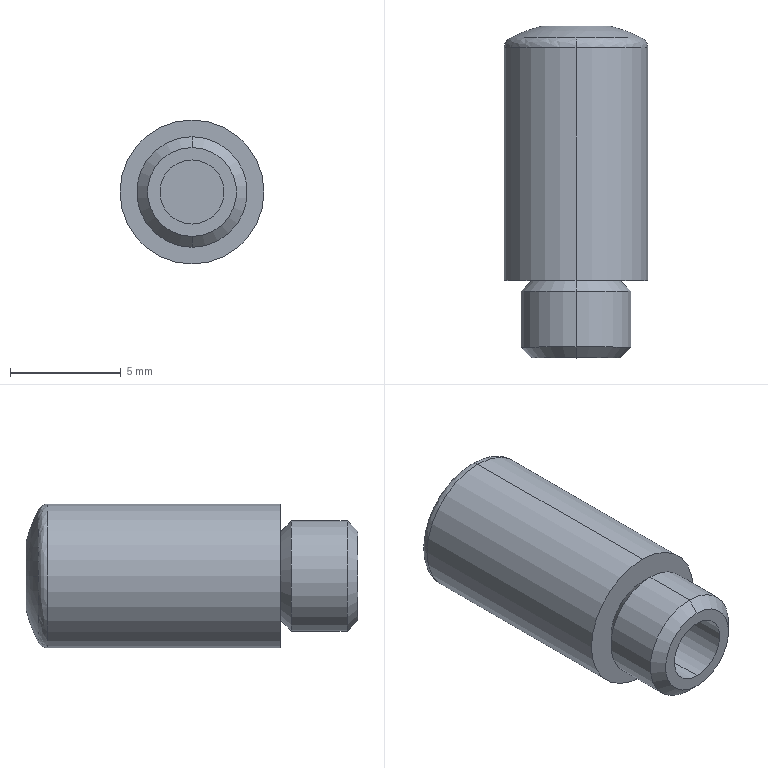Part | SolidWorks | features BaseBody 1 | 1 solid | 18 faces | box 6.5 x 15 x 6.5 mm | volume 404.686 mm3 | cylinder 6 | spline 4 | cone 4 | plane 4 | commonest cylinder face diameters 2.9 x2 5 x2 6.5 x2
STEP:
#1=CARTESIAN_POINT('',(-2.979,10.957,0.));
#2=VERTEX_POINT('',#1);
#3=CARTESIAN_POINT('',(0.,10.957,-2.979));
#4=VERTEX_POINT('',#3);
#5=CARTESIAN_POINT('',(0.,10.957,0.));
#6=DIRECTION('',(0.,-1.,0.));
#7=DIRECTION('',(0.,0.,1.));
#8=AXIS2_PLACEMENT_3D('',#5,#6,#7);
#9=CIRCLE('',#8,2.979);
#10=EDGE_CURVE('',#2,#4,#9,.T.);
#11=ORIENTED_EDGE('',*,*,#10,.T.);
#12=CARTESIAN_POINT('',(0.,10.513,-3.25));
#13=VERTEX_POINT('',#12);
#14=CARTESIAN_POINT('',(0.,10.513,-2.75));
#15=DIRECTION('',(-1.,0.,0.));
#16=DIRECTION('',(0.,0.,-1.));
#17=AXIS2_PLACEMENT_3D('',#14,#15,#16);
#18=CIRCLE('',#17,0.5);
#19=EDGE_CURVE('',#4,#13,#18,.T.);
#20=ORIENTED_EDGE('',*,*,#19,.T.);
#21=CARTESIAN_POINT('',(0.,10.513,3.25));
#22=VERTEX_POINT('',#21);
#23=CARTESIAN_POINT('',(0.,10.513,0.));
#24=DIRECTION('',(0.,-1.,0.));
#25=DIRECTION('',(0.,0.,-1.));
#26=AXIS2_PLACEMENT_3D('',#23,#24,#25);
#27=CIRCLE('',#26,3.25);
#28=EDGE_CURVE('',#22,#13,#27,.T.);
#29=ORIENTED_EDGE('',*,*,#28,.F.);
#30=CARTESIAN_POINT('',(0.,10.957,2.979));
#31=VERTEX_POINT('',#30);
#32=CARTESIAN_POINT('',(0.,10.513,2.75));
#33=DIRECTION('',(1.,0.,0.));
#34=DIRECTION('',(0.,0.,1.));
#35=AXIS2_PLACEMENT_3D('',#32,#33,#34);
#36=CIRCLE('',#35,0.5);
#37=EDGE_CURVE('',#31,#22,#36,.T.);
#38=ORIENTED_EDGE('',*,*,#37,.F.);
#39=CARTESIAN_POINT('',(0.,10.957,0.));
#40=DIRECTION('',(0.,-1.,0.));
#41=DIRECTION('',(0.,0.,1.));
#42=AXIS2_PLACEMENT_3D('',#39,#40,#41);
#43=CIRCLE('',#42,2.979);
#44=EDGE_CURVE('',#31,#2,#43,.T.);
#45=ORIENTED_EDGE('',*,*,#44,.T.);
#46=EDGE_LOOP('',(#11,#20,#29,#38,#45));
#47=FACE_OUTER_BOUND('',#46,.T.);
#48=CARTESIAN_POINT('',(0.,10.957,-2.979));
#49=CARTESIAN_POINT('',(-5.958,10.957,-2.979));
#50=CARTESIAN_POINT('',(-5.958,10.957,2.979));
#51=CARTESIAN_POINT('',(0.,10.957,2.979));
#52=CARTESIAN_POINT('',(0.,10.869,-3.15));
#53=CARTESIAN_POINT('',(-6.3,10.869,-3.15));
#54=CARTESIAN_POINT('',(-6.3,10.869,3.15));
#55=CARTESIAN_POINT('',(0.,10.869,3.15));
#56=CARTESIAN_POINT('',(0.,10.705,-3.25));
#57=CARTESIAN_POINT('',(-6.5,10.705,-3.25));
#58=CARTESIAN_POINT('',(-6.5,10.705,3.25));
#59=CARTESIAN_POINT('',(0.,10.705,3.25));
#60=CARTESIAN_POINT('',(0.,10.513,-3.25));
#61=CARTESIAN_POINT('',(-6.5,10.513,-3.25));
#62=CARTESIAN_POINT('',(-6.5,10.513,3.25));
#63=CARTESIAN_POINT('',(0.,10.513,3.25));
#64=(BOUNDED_SURFACE()B_SPLINE_SURFACE(3,3,((#48,#49,#50,#51),(#52,#53,#54,#55),(#56,#57,#58,#59),(#60,#61,#62,#63)),.UNSPECIFIED.,.F.,.F.,.F.)B_SPLINE_SURFACE_WITH_KNOTS((4,4),(4,4),(0.,1.),(0.,1.),.UNSPECIFIED.)GEOMETRIC_REPRESENTATION_ITEM()RATIONAL_B_SPLINE_SURFACE(((1.,0.3333,0.3333,1.),(0.9026,0.3009,0.3009,0.9026),(0.9026,0.3009,0.3009,0.9026),(1.,0.3333,0.3333,1.)))REPRESENTATION_ITEM('')SURFACE());
#65=ADVANCED_FACE('',(#47),#64,.T.);
#66=CARTESIAN_POINT('',(2.979,10.957,0.));
#67=VERTEX_POINT('',#66);
#68=CARTESIAN_POINT('',(0.,10.957,0.));
#69=DIRECTION('',(0.,-1.,0.));
#70=DIRECTION('',(0.,0.,1.));
#71=AXIS2_PLACEMENT_3D('',#68,#69,#70);
#72=CIRCLE('',#71,2.979);
#73=EDGE_CURVE('',#67,#31,#72,.T.);
#74=ORIENTED_EDGE('',*,*,#73,.F.);
#75=CARTESIAN_POINT('',(1.519,11.5,0.));
#76=VERTEX_POINT('',#75);
#77=CARTESIAN_POINT('',(0.,5.18,0.));
#78=DIRECTION('',(0.,0.,1.));
#79=DIRECTION('',(1.,0.,0.));
#80=AXIS2_PLACEMENT_3D('',#77,#78,#79);
#81=CIRCLE('',#80,6.5);
#82=EDGE_CURVE('',#67,#76,#81,.T.);
#83=ORIENTED_EDGE('',*,*,#82,.T.);
#84=CARTESIAN_POINT('',(-1.519,11.5,0.));
#85=VERTEX_POINT('',#84);
#86=CARTESIAN_POINT('',(1.519,11.5,0.));
#87=CARTESIAN_POINT('',(1.519,11.5,0.1003));
#88=CARTESIAN_POINT('',(1.509,11.5,0.199));
#89=CARTESIAN_POINT('',(1.471,11.5,0.3931));
#90=CARTESIAN_POINT('',(1.441,11.5,0.4896));
#91=CARTESIAN_POINT('',(1.365,11.5,0.6736));
#92=CARTESIAN_POINT('',(1.319,11.5,0.7608));
#93=CARTESIAN_POINT('',(1.208,11.5,0.9259));
#94=CARTESIAN_POINT('',(1.144,11.5,1.004));
#95=CARTESIAN_POINT('',(0.934,11.5,1.214));
#96=CARTESIAN_POINT('',(0.7645,11.5,1.327));
#97=CARTESIAN_POINT('',(0.399,11.5,1.479));
#98=CARTESIAN_POINT('',(0.1991,11.5,1.519));
#99=CARTESIAN_POINT('',(-0.09803,11.5,1.519));
#100=CARTESIAN_POINT('',(-0.1986,11.5,1.509));
#101=CARTESIAN_POINT('',(-0.3935,11.5,1.471));
#102=CARTESIAN_POINT('',(-0.4882,11.5,1.442));
#103=CARTESIAN_POINT('',(-0.6721,11.5,1.366));
#104=CARTESIAN_POINT('',(-0.761,11.5,1.318));
#105=CARTESIAN_POINT('',(-0.9257,11.5,1.209));
#106=CARTESIAN_POINT('',(-1.002,11.5,1.146));
#107=CARTESIAN_POINT('',(-1.215,11.5,0.9333));
#108=CARTESIAN_POINT('',(-1.327,11.5,0.7661));
#109=CARTESIAN_POINT('',(-1.479,11.5,0.398));
#110=CARTESIAN_POINT('',(-1.519,11.5,0.2007));
#111=CARTESIAN_POINT('',(-1.519,11.5,0.));
#112=B_SPLINE_CURVE_WITH_KNOTS('',3,(#86,#87,#88,#89,#90,#91,#92,#93,#94,#95,#96,#97,#98,#99,#100,#101,#102,#103,#104,#105,#106,#107,#108,#109,#110,#111),.UNSPECIFIED.,.F.,.F.,(4,2,2,2,2,2,2,2,2,2,2,2,4),(0.,0.0002968,0.0005935,0.0008903,0.001187,0.001781,0.002374,0.002671,0.002968,0.003264,0.003561,0.004155,0.004748),.UNSPECIFIED.);
#113=EDGE_CURVE('',#76,#85,#112,.T.);
#114=ORIENTED_EDGE('',*,*,#113,.T.);
#115=CARTESIAN_POINT('',(0.,5.18,0.));
#116=DIRECTION('',(0.,0.,1.));
#117=DIRECTION('',(1.,0.,0.));
#118=AXIS2_PLACEMENT_3D('',#115,#116,#117);
#119=CIRCLE('',#118,6.5);
#120=EDGE_CURVE('',#85,#2,#119,.T.);
#121=ORIENTED_EDGE('',*,*,#120,.T.);
#122=ORIENTED_EDGE('',*,*,#44,.F.);
#123=EDGE_LOOP('',(#74,#83,#114,#121,#122));
#124=FACE_OUTER_BOUND('',#123,.T.);
#125=CARTESIAN_POINT('',(3.012,10.94,0.));
#126=CARTESIAN_POINT('',(3.012,10.94,0.9285));
#127=CARTESIAN_POINT('',(3.012,10.72,1.831));
#128=CARTESIAN_POINT('',(3.012,10.292,2.655));
#129=CARTESIAN_POINT('',(1.087,11.947,0.));
#130=CARTESIAN_POINT('',(1.087,11.947,1.091));
#131=CARTESIAN_POINT('',(1.087,11.688,2.151));
#132=CARTESIAN_POINT('',(1.087,11.185,3.119));
#133=CARTESIAN_POINT('',(-1.087,11.947,0.));
#134=CARTESIAN_POINT('',(-1.087,11.947,1.091));
#135=CARTESIAN_POINT('',(-1.087,11.688,2.151));
#136=CARTESIAN_POINT('',(-1.087,11.185,3.119));
#137=CARTESIAN_POINT('',(-3.012,10.94,0.));
#138=CARTESIAN_POINT('',(-3.012,10.94,0.9285));
#139=CARTESIAN_POINT('',(-3.012,10.72,1.831));
#140=CARTESIAN_POINT('',(-3.012,10.292,2.655));
#141=(BOUNDED_SURFACE()B_SPLINE_SURFACE(3,3,((#125,#126,#127,#128),(#129,#130,#131,#132),(#133,#134,#135,#136),(#137,#138,#139,#140)),.UNSPECIFIED.,.F.,.F.,.F.)B_SPLINE_SURFACE_WITH_KNOTS((4,4),(4,4),(0.,1.),(0.,1.),.UNSPECIFIED.)GEOMETRIC_REPRESENTATION_ITEM()RATIONAL_B_SPLINE_SURFACE(((1.,0.981,0.981,1.),(0.9241,0.9065,0.9065,0.9241),(0.9241,0.9065,0.9065,0.9241),(1.,0.981,0.981,1.)))REPRESENTATION_ITEM('')SURFACE());
#142=ADVANCED_FACE('',(#124),#141,.T.);
#143=CARTESIAN_POINT('',(0.,10.513,0.));
#144=DIRECTION('',(0.,-1.,0.));
#145=DIRECTION('',(0.,0.,-1.));
#146=AXIS2_PLACEMENT_3D('',#143,#144,#145);
#147=CIRCLE('',#146,3.25);
#148=EDGE_CURVE('',#13,#22,#147,.T.);
#149=ORIENTED_EDGE('',*,*,#148,.T.);
#150=CARTESIAN_POINT('',(0.,0.,3.25));
#151=VERTEX_POINT('',#150);
#152=CARTESIAN_POINT('',(0.,5.256,3.25));
#153=DIRECTION('',(0.,-1.,0.));
#154=VECTOR('',#153,1000.);
#155=LINE('',#152,#154);
#156=EDGE_CURVE('',#22,#151,#155,.T.);
#157=ORIENTED_EDGE('',*,*,#156,.T.);
#158=CARTESIAN_POINT('',(0.,0.,-3.25));
#159=VERTEX_POINT('',#158);
#160=CARTESIAN_POINT('',(0.,0.,0.));
#161=DIRECTION('',(0.,1.,0.));
#162=DIRECTION('',(0.,0.,-1.));
#163=AXIS2_PLACEMENT_3D('',#160,#161,#162);
#164=CIRCLE('',#163,3.25);
#165=EDGE_CURVE('',#151,#159,#164,.T.);
#166=ORIENTED_EDGE('',*,*,#165,.T.);
#167=CARTESIAN_POINT('',(0.,5.256,-3.25));
#168=DIRECTION('',(0.,-1.,0.));
#169=VECTOR('',#168,1000.);
#170=LINE('',#167,#169);
#171=EDGE_CURVE('',#13,#159,#170,.T.);
#172=ORIENTED_EDGE('',*,*,#171,.F.);
#173=EDGE_LOOP('',(#149,#157,#166,#172));
#174=FACE_OUTER_BOUND('',#173,.T.);
#175=CARTESIAN_POINT('',(0.,5.256,0.));
#176=DIRECTION('',(0.,-1.,0.));
#177=DIRECTION('',(0.,0.,-1.));
#178=AXIS2_PLACEMENT_3D('',#175,#176,#177);
#179=CYLINDRICAL_SURFACE('',#178,3.25);
#180=ADVANCED_FACE('',(#174),#179,.T.);
#181=CARTESIAN_POINT('',(0.,0.,2.009));
#182=VERTEX_POINT('',#181);
#183=CARTESIAN_POINT('',(0.,0.,-2.009));
#184=VERTEX_POINT('',#183);
#185=CARTESIAN_POINT('',(0.,0.,0.));
#186=DIRECTION('',(0.,1.,0.));
#187=DIRECTION('',(0.,0.,-1.));
#188=AXIS2_PLACEMENT_3D('',#185,#186,#187);
#189=CIRCLE('',#188,2.009);
#190=EDGE_CURVE('',#182,#184,#189,.T.);
#191=ORIENTED_EDGE('',*,*,#190,.F.);
#192=CARTESIAN_POINT('',(0.,-0.4905,2.5));
#193=VERTEX_POINT('',#192);
#194=CARTESIAN_POINT('',(0.,-0.4905,2.5));
#195=DIRECTION('',(0.,-0.7071,0.7071));
#196=VECTOR('',#195,1000.);
#197=LINE('',#194,#196);
#198=EDGE_CURVE('',#182,#193,#197,.T.);
#199=ORIENTED_EDGE('',*,*,#198,.T.);
#200=CARTESIAN_POINT('',(0.,-0.4905,-2.5));
#201=VERTEX_POINT('',#200);
#202=CARTESIAN_POINT('',(0.,-0.4905,0.));
#203=DIRECTION('',(0.,1.,0.));
#204=DIRECTION('',(1.,0.,0.));
#205=AXIS2_PLACEMENT_3D('',#202,#203,#204);
#206=CIRCLE('',#205,2.5);
#207=EDGE_CURVE('',#193,#201,#206,.T.);
#208=ORIENTED_EDGE('',*,*,#207,.T.);
#209=CARTESIAN_POINT('',(0.,-0.4905,-2.5));
#210=DIRECTION('',(0.,-0.7071,-0.7071));
#211=VECTOR('',#210,1000.);
#212=LINE('',#209,#211);
#213=EDGE_CURVE('',#184,#201,#212,.T.);
#214=ORIENTED_EDGE('',*,*,#213,.F.);
#215=EDGE_LOOP('',(#191,#199,#208,#214));
#216=FACE_OUTER_BOUND('',#215,.T.);
#217=CARTESIAN_POINT('',(0.,-0.4905,0.));
#218=DIRECTION('',(0.,-1.,0.));
#219=DIRECTION('',(0.,0.,-1.));
#220=AXIS2_PLACEMENT_3D('',#217,#218,#219);
#221=CONICAL_SURFACE('',#220,2.5,0.7854);
#222=ADVANCED_FACE('',(#216),#221,.T.);
#223=ORIENTED_EDGE('',*,*,#207,.F.);
#224=CARTESIAN_POINT('',(0.,-3.01,2.5));
#225=VERTEX_POINT('',#224);
#226=CARTESIAN_POINT('',(0.,-1.75,2.5));
#227=DIRECTION('',(0.,-1.,0.));
#228=VECTOR('',#227,1000.);
#229=LINE('',#226,#228);
#230=EDGE_CURVE('',#193,#225,#229,.T.);
#231=ORIENTED_EDGE('',*,*,#230,.T.);
#232=CARTESIAN_POINT('',(0.,-3.01,-2.5));
#233=VERTEX_POINT('',#232);
#234=CARTESIAN_POINT('',(0.,-3.01,0.));
#235=DIRECTION('',(0.,1.,0.));
#236=DIRECTION('',(0.,0.,-1.));
#237=AXIS2_PLACEMENT_3D('',#234,#235,#236);
#238=CIRCLE('',#237,2.5);
#239=EDGE_CURVE('',#225,#233,#238,.T.);
#240=ORIENTED_EDGE('',*,*,#239,.T.);
#241=CARTESIAN_POINT('',(0.,-1.75,-2.5));
#242=DIRECTION('',(0.,-1.,0.));
#243=VECTOR('',#242,1000.);
#244=LINE('',#241,#243);
#245=EDGE_CURVE('',#201,#233,#244,.T.);
#246=ORIENTED_EDGE('',*,*,#245,.F.);
#247=EDGE_LOOP('',(#223,#231,#240,#246));
#248=FACE_OUTER_BOUND('',#247,.T.);
#249=CARTESIAN_POINT('',(0.,-1.75,0.));
#250=DIRECTION('',(0.,-1.,0.));
#251=DIRECTION('',(0.,0.,-1.));
#252=AXIS2_PLACEMENT_3D('',#249,#250,#251);
#253=CYLINDRICAL_SURFACE('',#252,2.5);
#254=ADVANCED_FACE('',(#248),#253,.T.);
#255=CARTESIAN_POINT('',(0.,-3.5,2.01));
#256=VERTEX_POINT('',#255);
#257=CARTESIAN_POINT('',(0.,-3.5,-2.01));
#258=VERTEX_POINT('',#257);
#259=CARTESIAN_POINT('',(0.,-3.5,0.));
#260=DIRECTION('',(0.,1.,0.));
#261=DIRECTION('',(0.,0.,1.));
#262=AXIS2_PLACEMENT_3D('',#259,#260,#261);
#263=CIRCLE('',#262,2.01);
#264=EDGE_CURVE('',#256,#258,#263,.T.);
#265=ORIENTED_EDGE('',*,*,#264,.T.);
#266=CARTESIAN_POINT('',(0.,-3.009,-2.5));
#267=DIRECTION('',(0.,0.7071,-0.7071));
#268=VECTOR('',#267,1000.);
#269=LINE('',#266,#268);
#270=EDGE_CURVE('',#258,#233,#269,.T.);
#271=ORIENTED_EDGE('',*,*,#270,.T.);
#272=ORIENTED_EDGE('',*,*,#239,.F.);
#273=CARTESIAN_POINT('',(0.,-3.009,2.5));
#274=DIRECTION('',(0.,0.7071,0.7071));
#275=VECTOR('',#274,1000.);
#276=LINE('',#273,#275);
#277=EDGE_CURVE('',#256,#225,#276,.T.);
#278=ORIENTED_EDGE('',*,*,#277,.F.);
#279=EDGE_LOOP('',(#265,#271,#272,#278));
#280=FACE_OUTER_BOUND('',#279,.T.);
#281=CARTESIAN_POINT('',(0.,-3.009,0.));
#282=DIRECTION('',(0.,1.,0.));
#283=DIRECTION('',(0.,0.,1.));
#284=AXIS2_PLACEMENT_3D('',#281,#282,#283);
#285=CONICAL_SURFACE('',#284,2.5,0.7854);
#286=ADVANCED_FACE('',(#280),#285,.T.);
#287=CARTESIAN_POINT('',(0.,1.5,1.45));
#288=VERTEX_POINT('',#287);
#289=CARTESIAN_POINT('',(0.,1.5,-1.45));
#290=VERTEX_POINT('',#289);
#291=CARTESIAN_POINT('',(0.,1.5,0.));
#292=DIRECTION('',(0.,-1.,0.));
#293=DIRECTION('',(0.,0.,-1.));
#294=AXIS2_PLACEMENT_3D('',#291,#292,#293);
#295=CIRCLE('',#294,1.45);
#296=EDGE_CURVE('',#288,#290,#295,.T.);
#297=ORIENTED_EDGE('',*,*,#296,.F.);
#298=CARTESIAN_POINT('',(0.,-3.5,1.45));
#299=VERTEX_POINT('',#298);
#300=CARTESIAN_POINT('',(0.,-1.,1.45));
#301=DIRECTION('',(0.,-1.,0.));
#302=VECTOR('',#301,1000.);
#303=LINE('',#300,#302);
#304=EDGE_CURVE('',#288,#299,#303,.T.);
#305=ORIENTED_EDGE('',*,*,#304,.T.);
#306=CARTESIAN_POINT('',(0.,-3.5,-1.45));
#307=VERTEX_POINT('',#306);
#308=CARTESIAN_POINT('',(0.,-3.5,0.));
#309=DIRECTION('',(0.,1.,0.));
#310=DIRECTION('',(0.,0.,-1.));
#311=AXIS2_PLACEMENT_3D('',#308,#309,#310);
#312=CIRCLE('',#311,1.45);
#313=EDGE_CURVE('',#307,#299,#312,.T.);
#314=ORIENTED_EDGE('',*,*,#313,.F.);
#315=CARTESIAN_POINT('',(0.,-1.,-1.45));
#316=DIRECTION('',(0.,-1.,0.));
#317=VECTOR('',#316,1000.);
#318=LINE('',#315,#317);
#319=EDGE_CURVE('',#290,#307,#318,.T.);
#320=ORIENTED_EDGE('',*,*,#319,.F.);
#321=EDGE_LOOP('',(#297,#305,#314,#320));
#322=FACE_OUTER_BOUND('',#321,.T.);
#323=CARTESIAN_POINT('',(0.,-1.,0.));
#324=DIRECTION('',(0.,-1.,0.));
#325=DIRECTION('',(0.,0.,-1.));
#326=AXIS2_PLACEMENT_3D('',#323,#324,#325);
#327=CYLINDRICAL_SURFACE('',#326,1.45);
#328=ADVANCED_FACE('',(#322),#327,.F.);
#329=ORIENTED_EDGE('',*,*,#156,.F.);
#330=ORIENTED_EDGE('',*,*,#28,.T.);
#331=ORIENTED_EDGE('',*,*,#171,.T.);
#332=CARTESIAN_POINT('',(0.,0.,0.));
#333=DIRECTION('',(0.,1.,0.));
#334=DIRECTION('',(0.,0.,-1.));
#335=AXIS2_PLACEMENT_3D('',#332,#333,#334);
#336=CIRCLE('',#335,3.25);
#337=EDGE_CURVE('',#159,#151,#336,.T.);
#338=ORIENTED_EDGE('',*,*,#337,.T.);
#339=EDGE_LOOP('',(#329,#330,#331,#338));
#340=FACE_OUTER_BOUND('',#339,.T.);
#341=CARTESIAN_POINT('',(0.,5.256,0.));
#342=DIRECTION('',(0.,-1.,0.));
#343=DIRECTION('',(0.,0.,-1.));
#344=AXIS2_PLACEMENT_3D('',#341,#342,#343);
#345=CYLINDRICAL_SURFACE('',#344,3.25);
#346=ADVANCED_FACE('',(#340),#345,.T.);
#347=ORIENTED_EDGE('',*,*,#19,.F.);
#348=CARTESIAN_POINT('',(0.,10.957,0.));
#349=DIRECTION('',(0.,-1.,0.));
#350=DIRECTION('',(0.,0.,1.));
#351=AXIS2_PLACEMENT_3D('',#348,#349,#350);
#352=CIRCLE('',#351,2.979);
#353=EDGE_CURVE('',#4,#67,#352,.T.);
#354=ORIENTED_EDGE('',*,*,#353,.T.);
#355=ORIENTED_EDGE('',*,*,#73,.T.);
#356=ORIENTED_EDGE('',*,*,#37,.T.);
#357=ORIENTED_EDGE('',*,*,#148,.F.);
#358=EDGE_LOOP('',(#347,#354,#355,#356,#357));
#359=FACE_OUTER_BOUND('',#358,.T.);
#360=CARTESIAN_POINT('',(0.,10.957,2.979));
#361=CARTESIAN_POINT('',(5.958,10.957,2.979));
#362=CARTESIAN_POINT('',(5.958,10.957,-2.979));
#363=CARTESIAN_POINT('',(0.,10.957,-2.979));
#364=CARTESIAN_POINT('',(0.,10.869,3.15));
#365=CARTESIAN_POINT('',(6.3,10.869,3.15));
#366=CARTESIAN_POINT('',(6.3,10.869,-3.15));
#367=CARTESIAN_POINT('',(0.,10.869,-3.15));
#368=CARTESIAN_POINT('',(0.,10.705,3.25));
#369=CARTESIAN_POINT('',(6.5,10.705,3.25));
#370=CARTESIAN_POINT('',(6.5,10.705,-3.25));
#371=CARTESIAN_POINT('',(0.,10.705,-3.25));
#372=CARTESIAN_POINT('',(0.,10.513,3.25));
#373=CARTESIAN_POINT('',(6.5,10.513,3.25));
#374=CARTESIAN_POINT('',(6.5,10.513,-3.25));
#375=CARTESIAN_POINT('',(0.,10.513,-3.25));
#376=(BOUNDED_SURFACE()B_SPLINE_SURFACE(3,3,((#360,#361,#362,#363),(#364,#365,#366,#367),(#368,#369,#370,#371),(#372,#373,#374,#375)),.UNSPECIFIED.,.F.,.F.,.T.)B_SPLINE_SURFACE_WITH_KNOTS((4,4),(4,4),(0.,1.),(0.,1.),.UNSPECIFIED.)GEOMETRIC_REPRESENTATION_ITEM()RATIONAL_B_SPLINE_SURFACE(((1.,0.3333,0.3333,1.),(0.9026,0.3009,0.3009,0.9026),(0.9026,0.3009,0.3009,0.9026),(1.,0.3333,0.3333,1.)))REPRESENTATION_ITEM('')SURFACE());
#377=ADVANCED_FACE('',(#359),#376,.T.);
#378=CARTESIAN_POINT('',(0.,0.,0.));
#379=DIRECTION('',(0.,1.,0.));
#380=DIRECTION('',(0.,0.,-1.));
#381=AXIS2_PLACEMENT_3D('',#378,#379,#380);
#382=CIRCLE('',#381,2.009);
#383=EDGE_CURVE('',#184,#182,#382,.T.);
#384=ORIENTED_EDGE('',*,*,#383,.T.);
#385=ORIENTED_EDGE('',*,*,#190,.T.);
#386=EDGE_LOOP('',(#384,#385));
#387=FACE_BOUND('',#386,.T.);
#388=ORIENTED_EDGE('',*,*,#337,.F.);
#389=ORIENTED_EDGE('',*,*,#165,.F.);
#390=EDGE_LOOP('',(#388,#389));
#391=FACE_OUTER_BOUND('',#390,.T.);
#392=CARTESIAN_POINT('',(2.63,0.,0.));
#393=DIRECTION('',(0.,-1.,0.));
#394=DIRECTION('',(0.,0.,-1.));
#395=AXIS2_PLACEMENT_3D('',#392,#393,#394);
#396=PLANE('',#395);
#397=ADVANCED_FACE('',(#387,#391),#396,.T.);
#398=ORIENTED_EDGE('',*,*,#82,.F.);
#399=ORIENTED_EDGE('',*,*,#353,.F.);
#400=ORIENTED_EDGE('',*,*,#10,.F.);
#401=ORIENTED_EDGE('',*,*,#120,.F.);
#402=CARTESIAN_POINT('',(-1.519,11.5,0.));
#403=CARTESIAN_POINT('',(-1.519,11.5,-0.1003));
#404=CARTESIAN_POINT('',(-1.509,11.5,-0.199));
#405=CARTESIAN_POINT('',(-1.471,11.5,-0.3931));
#406=CARTESIAN_POINT('',(-1.441,11.5,-0.4896));
#407=CARTESIAN_POINT('',(-1.365,11.5,-0.6736));
#408=CARTESIAN_POINT('',(-1.319,11.5,-0.7608));
#409=CARTESIAN_POINT('',(-1.208,11.5,-0.9259));
#410=CARTESIAN_POINT('',(-1.144,11.5,-1.004));
#411=CARTESIAN_POINT('',(-0.934,11.5,-1.214));
#412=CARTESIAN_POINT('',(-0.7645,11.5,-1.327));
#413=CARTESIAN_POINT('',(-0.399,11.5,-1.479));
#414=CARTESIAN_POINT('',(-0.1991,11.5,-1.519));
#415=CARTESIAN_POINT('',(0.09803,11.5,-1.519));
#416=CARTESIAN_POINT('',(0.1986,11.5,-1.509));
#417=CARTESIAN_POINT('',(0.3935,11.5,-1.471));
#418=CARTESIAN_POINT('',(0.4882,11.5,-1.442));
#419=CARTESIAN_POINT('',(0.6721,11.5,-1.366));
#420=CARTESIAN_POINT('',(0.761,11.5,-1.318));
#421=CARTESIAN_POINT('',(0.9257,11.5,-1.209));
#422=CARTESIAN_POINT('',(1.002,11.5,-1.146));
#423=CARTESIAN_POINT('',(1.215,11.5,-0.9333));
#424=CARTESIAN_POINT('',(1.327,11.5,-0.7661));
#425=CARTESIAN_POINT('',(1.479,11.5,-0.398));
#426=CARTESIAN_POINT('',(1.519,11.5,-0.2007));
#427=CARTESIAN_POINT('',(1.519,11.5,0.));
#428=B_SPLINE_CURVE_WITH_KNOTS('',3,(#402,#403,#404,#405,#406,#407,#408,#409,#410,#411,#412,#413,#414,#415,#416,#417,#418,#419,#420,#421,#422,#423,#424,#425,#426,#427),.UNSPECIFIED.,.F.,.F.,(4,2,2,2,2,2,2,2,2,2,2,2,4),(0.004748,0.005045,0.005342,0.005639,0.005935,0.006529,0.007123,0.007419,0.007716,0.008013,0.00831,0.008903,0.009497),.UNSPECIFIED.);
#429=EDGE_CURVE('',#85,#76,#428,.T.);
#430=ORIENTED_EDGE('',*,*,#429,.T.);
#431=EDGE_LOOP('',(#398,#399,#400,#401,#430));
#432=FACE_OUTER_BOUND('',#431,.T.);
#433=CARTESIAN_POINT('',(3.012,10.292,-2.655));
#434=CARTESIAN_POINT('',(3.012,10.72,-1.831));
#435=CARTESIAN_POINT('',(3.012,10.94,-0.9285));
#436=CARTESIAN_POINT('',(3.012,10.94,0.));
#437=CARTESIAN_POINT('',(1.087,11.185,-3.119));
#438=CARTESIAN_POINT('',(1.087,11.688,-2.151));
#439=CARTESIAN_POINT('',(1.087,11.947,-1.091));
#440=CARTESIAN_POINT('',(1.087,11.947,0.));
#441=CARTESIAN_POINT('',(-1.087,11.185,-3.119));
#442=CARTESIAN_POINT('',(-1.087,11.688,-2.151));
#443=CARTESIAN_POINT('',(-1.087,11.947,-1.091));
#444=CARTESIAN_POINT('',(-1.087,11.947,0.));
#445=CARTESIAN_POINT('',(-3.012,10.292,-2.655));
#446=CARTESIAN_POINT('',(-3.012,10.72,-1.831));
#447=CARTESIAN_POINT('',(-3.012,10.94,-0.9285));
#448=CARTESIAN_POINT('',(-3.012,10.94,0.));
#449=(BOUNDED_SURFACE()B_SPLINE_SURFACE(3,3,((#433,#434,#435,#436),(#437,#438,#439,#440),(#441,#442,#443,#444),(#445,#446,#447,#448)),.UNSPECIFIED.,.F.,.F.,.F.)B_SPLINE_SURFACE_WITH_KNOTS((4,4),(4,4),(0.,1.),(0.,1.),.UNSPECIFIED.)GEOMETRIC_REPRESENTATION_ITEM()RATIONAL_B_SPLINE_SURFACE(((1.,0.981,0.981,1.),(0.9241,0.9065,0.9065,0.9241),(0.9241,0.9065,0.9065,0.9241),(1.,0.981,0.981,1.)))REPRESENTATION_ITEM('')SURFACE());
#450=ADVANCED_FACE('',(#432),#449,.T.);
#451=ORIENTED_EDGE('',*,*,#198,.F.);
#452=ORIENTED_EDGE('',*,*,#383,.F.);
#453=ORIENTED_EDGE('',*,*,#213,.T.);
#454=CARTESIAN_POINT('',(0.,-0.4905,0.));
#455=DIRECTION('',(0.,1.,0.));
#456=DIRECTION('',(1.,0.,0.));
#457=AXIS2_PLACEMENT_3D('',#454,#455,#456);
#458=CIRCLE('',#457,2.5);
#459=EDGE_CURVE('',#201,#193,#458,.T.);
#460=ORIENTED_EDGE('',*,*,#459,.T.);
#461=EDGE_LOOP('',(#451,#452,#453,#460));
#462=FACE_OUTER_BOUND('',#461,.T.);
#463=CARTESIAN_POINT('',(0.,-0.4905,0.));
#464=DIRECTION('',(0.,-1.,0.));
#465=DIRECTION('',(0.,0.,-1.));
#466=AXIS2_PLACEMENT_3D('',#463,#464,#465);
#467=CONICAL_SURFACE('',#466,2.5,0.7854);
#468=ADVANCED_FACE('',(#462),#467,.T.);
#469=ORIENTED_EDGE('',*,*,#113,.F.);
#470=ORIENTED_EDGE('',*,*,#429,.F.);
#471=EDGE_LOOP('',(#469,#470));
#472=FACE_OUTER_BOUND('',#471,.T.);
#473=CARTESIAN_POINT('',(0.7595,11.5,0.));
#474=DIRECTION('',(0.,1.,0.));
#475=DIRECTION('',(0.,0.,1.));
#476=AXIS2_PLACEMENT_3D('',#473,#474,#475);
#477=PLANE('',#476);
#478=ADVANCED_FACE('',(#472),#477,.T.);
#479=ORIENTED_EDGE('',*,*,#230,.F.);
#480=ORIENTED_EDGE('',*,*,#459,.F.);
#481=ORIENTED_EDGE('',*,*,#245,.T.);
#482=CARTESIAN_POINT('',(0.,-3.01,0.));
#483=DIRECTION('',(0.,1.,0.));
#484=DIRECTION('',(0.,0.,-1.));
#485=AXIS2_PLACEMENT_3D('',#482,#483,#484);
#486=CIRCLE('',#485,2.5);
#487=EDGE_CURVE('',#233,#225,#486,.T.);
#488=ORIENTED_EDGE('',*,*,#487,.T.);
#489=EDGE_LOOP('',(#479,#480,#481,#488));
#490=FACE_OUTER_BOUND('',#489,.T.);
#491=CARTESIAN_POINT('',(0.,-1.75,0.));
#492=DIRECTION('',(0.,-1.,0.));
#493=DIRECTION('',(0.,0.,-1.));
#494=AXIS2_PLACEMENT_3D('',#491,#492,#493);
#495=CYLINDRICAL_SURFACE('',#494,2.5);
#496=ADVANCED_FACE('',(#490),#495,.T.);
#497=ORIENTED_EDGE('',*,*,#270,.F.);
#498=CARTESIAN_POINT('',(0.,-3.5,0.));
#499=DIRECTION('',(0.,1.,0.));
#500=DIRECTION('',(0.,0.,1.));
#501=AXIS2_PLACEMENT_3D('',#498,#499,#500);
#502=CIRCLE('',#501,2.01);
#503=EDGE_CURVE('',#258,#256,#502,.T.);
#504=ORIENTED_EDGE('',*,*,#503,.T.);
#505=ORIENTED_EDGE('',*,*,#277,.T.);
#506=ORIENTED_EDGE('',*,*,#487,.F.);
#507=EDGE_LOOP('',(#497,#504,#505,#506));
#508=FACE_OUTER_BOUND('',#507,.T.);
#509=CARTESIAN_POINT('',(0.,-3.009,0.));
#510=DIRECTION('',(0.,1.,0.));
#511=DIRECTION('',(0.,0.,1.));
#512=AXIS2_PLACEMENT_3D('',#509,#510,#511);
#513=CONICAL_SURFACE('',#512,2.5,0.7854);
#514=ADVANCED_FACE('',(#508),#513,.T.);
#515=ORIENTED_EDGE('',*,*,#313,.T.);
#516=CARTESIAN_POINT('',(0.,-3.5,0.));
#517=DIRECTION('',(0.,1.,0.));
#518=DIRECTION('',(0.,0.,-1.));
#519=AXIS2_PLACEMENT_3D('',#516,#517,#518);
#520=CIRCLE('',#519,1.45);
#521=EDGE_CURVE('',#299,#307,#520,.T.);
#522=ORIENTED_EDGE('',*,*,#521,.T.);
#523=EDGE_LOOP('',(#515,#522));
#524=FACE_BOUND('',#523,.T.);
#525=ORIENTED_EDGE('',*,*,#264,.F.);
#526=ORIENTED_EDGE('',*,*,#503,.F.);
#527=EDGE_LOOP('',(#525,#526));
#528=FACE_OUTER_BOUND('',#527,.T.);
#529=CARTESIAN_POINT('',(1.73,-3.5,0.));
#530=DIRECTION('',(0.,-1.,0.));
#531=DIRECTION('',(0.,0.,-1.));
#532=AXIS2_PLACEMENT_3D('',#529,#530,#531);
#533=PLANE('',#532);
#534=ADVANCED_FACE('',(#524,#528),#533,.T.);
#535=ORIENTED_EDGE('',*,*,#304,.F.);
#536=CARTESIAN_POINT('',(0.,1.5,0.));
#537=DIRECTION('',(0.,-1.,0.));
#538=DIRECTION('',(0.,0.,-1.));
#539=AXIS2_PLACEMENT_3D('',#536,#537,#538);
#540=CIRCLE('',#539,1.45);
#541=EDGE_CURVE('',#290,#288,#540,.T.);
#542=ORIENTED_EDGE('',*,*,#541,.F.);
#543=ORIENTED_EDGE('',*,*,#319,.T.);
#544=ORIENTED_EDGE('',*,*,#521,.F.);
#545=EDGE_LOOP('',(#535,#542,#543,#544));
#546=FACE_OUTER_BOUND('',#545,.T.);
#547=CARTESIAN_POINT('',(0.,-1.,0.));
#548=DIRECTION('',(0.,-1.,0.));
#549=DIRECTION('',(0.,0.,-1.));
#550=AXIS2_PLACEMENT_3D('',#547,#548,#549);
#551=CYLINDRICAL_SURFACE('',#550,1.45);
#552=ADVANCED_FACE('',(#546),#551,.F.);
#553=ORIENTED_EDGE('',*,*,#541,.T.);
#554=ORIENTED_EDGE('',*,*,#296,.T.);
#555=EDGE_LOOP('',(#553,#554));
#556=FACE_OUTER_BOUND('',#555,.T.);
#557=CARTESIAN_POINT('',(0.725,1.5,0.));
#558=DIRECTION('',(0.,-1.,0.));
#559=DIRECTION('',(0.,0.,-1.));
#560=AXIS2_PLACEMENT_3D('',#557,#558,#559);
#561=PLANE('',#560);
#562=ADVANCED_FACE('',(#556),#561,.T.);
#563=CLOSED_SHELL('',(#65,#142,#180,#222,#254,#286,#328,#346,#377,#397,#450,#468,#478,#496,#514,#534,#552,#562));
#564=MANIFOLD_SOLID_BREP('',#563);
#565=CARTESIAN_POINT('',(0.,0.,0.));
#566=DIRECTION('',(0.,0.,1.));
#567=DIRECTION('',(1.,0.,0.));
#568=AXIS2_PLACEMENT_3D('',#565,#566,#567);
#569=(LENGTH_UNIT()NAMED_UNIT(*)SI_UNIT(.MILLI.,.METRE.));
#570=UNCERTAINTY_MEASURE_WITH_UNIT(LENGTH_MEASURE(0.00001),#569,'','');
#571=(NAMED_UNIT(*)PLANE_ANGLE_UNIT()SI_UNIT($,.RADIAN.));
#572=(NAMED_UNIT(*)SI_UNIT($,.STERADIAN.)SOLID_ANGLE_UNIT());
#573=(GEOMETRIC_REPRESENTATION_CONTEXT(3)GLOBAL_UNCERTAINTY_ASSIGNED_CONTEXT((#570))GLOBAL_UNIT_ASSIGNED_CONTEXT((#569,#571,#572))REPRESENTATION_CONTEXT('',''));
#574=ADVANCED_BREP_SHAPE_REPRESENTATION('',(#564,#568),#573);